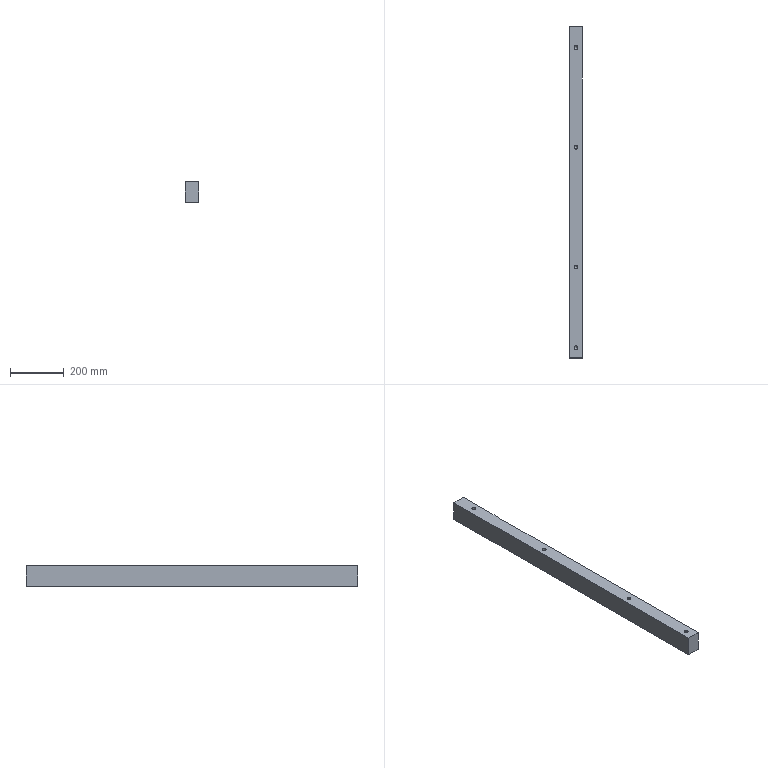Part | NX | features 3 2 | 1 solid | 24 faces | box 50 x 1233 x 75.5 mm | volume 4639640 mm3 | cylinder 9 | cone 8 | plane 7 | commonest cylinder face diameters 14.1 x8 54 x1
STEP:
#1=CARTESIAN_POINT('',(937.05,-522.5,256.5));
#2=VERTEX_POINT('',#1);
#3=CARTESIAN_POINT('',(930.,-522.5,256.5));
#4=DIRECTION('',(0.,0.,-1.));
#5=DIRECTION('',(1.,0.,0.));
#6=AXIS2_PLACEMENT_3D('',#3,#4,#5);
#7=CIRCLE('',#6,7.05);
#8=EDGE_CURVE('',#2,#2,#7,.T.);
#9=ORIENTED_EDGE('',*,*,#8,.T.);
#10=EDGE_LOOP('',(#9));
#11=FACE_BOUND('',#10,.T.);
#12=CARTESIAN_POINT('',(937.05,222.5,256.5));
#13=VERTEX_POINT('',#12);
#14=CARTESIAN_POINT('',(930.,222.5,256.5));
#15=DIRECTION('',(0.,0.,-1.));
#16=DIRECTION('',(1.,0.,0.));
#17=AXIS2_PLACEMENT_3D('',#14,#15,#16);
#18=CIRCLE('',#17,7.05);
#19=EDGE_CURVE('',#13,#13,#18,.T.);
#20=ORIENTED_EDGE('',*,*,#19,.T.);
#21=EDGE_LOOP('',(#20));
#22=FACE_BOUND('',#21,.T.);
#23=CARTESIAN_POINT('',(955.,469.802,256.5));
#24=VERTEX_POINT('',#23);
#25=CARTESIAN_POINT('',(955.,490.198,256.5));
#26=VERTEX_POINT('',#25);
#27=CARTESIAN_POINT('',(980.,480.,256.5));
#28=DIRECTION('',(0.,0.,-1.));
#29=DIRECTION('',(1.,0.,0.));
#30=AXIS2_PLACEMENT_3D('',#27,#28,#29);
#31=CIRCLE('',#30,27.);
#32=EDGE_CURVE('',#24,#26,#31,.T.);
#33=ORIENTED_EDGE('',*,*,#32,.T.);
#34=CARTESIAN_POINT('',(955.,672.5,256.5));
#35=VERTEX_POINT('',#34);
#36=CARTESIAN_POINT('',(955.,193.,256.5));
#37=DIRECTION('',(0.,-1.,0.));
#38=VECTOR('',#37,1000.);
#39=LINE('',#36,#38);
#40=EDGE_CURVE('',#35,#26,#39,.T.);
#41=ORIENTED_EDGE('',*,*,#40,.F.);
#42=CARTESIAN_POINT('',(905.,672.5,256.5));
#43=VERTEX_POINT('',#42);
#44=CARTESIAN_POINT('',(905.,672.5,256.5));
#45=DIRECTION('',(1.,0.,0.));
#46=VECTOR('',#45,1000.);
#47=LINE('',#44,#46);
#48=EDGE_CURVE('',#43,#35,#47,.T.);
#49=ORIENTED_EDGE('',*,*,#48,.F.);
#50=CARTESIAN_POINT('',(905.,-560.5,256.5));
#51=VERTEX_POINT('',#50);
#52=CARTESIAN_POINT('',(905.,193.,256.5));
#53=DIRECTION('',(0.,1.,0.));
#54=VECTOR('',#53,1000.);
#55=LINE('',#52,#54);
#56=EDGE_CURVE('',#51,#43,#55,.T.);
#57=ORIENTED_EDGE('',*,*,#56,.F.);
#58=CARTESIAN_POINT('',(955.,-560.5,256.5));
#59=VERTEX_POINT('',#58);
#60=CARTESIAN_POINT('',(2945.,-560.5,256.5));
#61=DIRECTION('',(1.,0.,0.));
#62=VECTOR('',#61,1000.);
#63=LINE('',#60,#62);
#64=EDGE_CURVE('',#51,#59,#63,.T.);
#65=ORIENTED_EDGE('',*,*,#64,.T.);
#66=CARTESIAN_POINT('',(955.,193.,256.5));
#67=DIRECTION('',(0.,-1.,0.));
#68=VECTOR('',#67,1000.);
#69=LINE('',#66,#68);
#70=EDGE_CURVE('',#24,#59,#69,.T.);
#71=ORIENTED_EDGE('',*,*,#70,.F.);
#72=EDGE_LOOP('',(#33,#41,#49,#57,#65,#71));
#73=FACE_BOUND('',#72,.T.);
#74=CARTESIAN_POINT('',(937.05,-222.5,256.5));
#75=VERTEX_POINT('',#74);
#76=CARTESIAN_POINT('',(930.,-222.5,256.5));
#77=DIRECTION('',(0.,0.,-1.));
#78=DIRECTION('',(1.,0.,0.));
#79=AXIS2_PLACEMENT_3D('',#76,#77,#78);
#80=CIRCLE('',#79,7.05);
#81=EDGE_CURVE('',#75,#75,#80,.T.);
#82=ORIENTED_EDGE('',*,*,#81,.T.);
#83=EDGE_LOOP('',(#82));
#84=FACE_BOUND('',#83,.T.);
#85=CARTESIAN_POINT('',(937.05,592.5,256.5));
#86=VERTEX_POINT('',#85);
#87=CARTESIAN_POINT('',(930.,592.5,256.5));
#88=DIRECTION('',(0.,0.,-1.));
#89=DIRECTION('',(1.,0.,0.));
#90=AXIS2_PLACEMENT_3D('',#87,#88,#89);
#91=CIRCLE('',#90,7.05);
#92=EDGE_CURVE('',#86,#86,#91,.T.);
#93=ORIENTED_EDGE('',*,*,#92,.T.);
#94=EDGE_LOOP('',(#93));
#95=FACE_BOUND('',#94,.T.);
#96=CARTESIAN_POINT('',(2945.,0.,256.5));
#97=DIRECTION('',(0.,0.,1.));
#98=DIRECTION('',(-1.,0.,0.));
#99=AXIS2_PLACEMENT_3D('',#96,#97,#98);
#100=PLANE('',#99);
#101=ADVANCED_FACE('',(#11,#22,#73,#84,#95),#100,.T.);
#102=CARTESIAN_POINT('',(937.05,222.5,181.));
#103=VERTEX_POINT('',#102);
#104=CARTESIAN_POINT('',(930.,222.5,181.));
#105=DIRECTION('',(0.,0.,1.));
#106=DIRECTION('',(1.,0.,0.));
#107=AXIS2_PLACEMENT_3D('',#104,#105,#106);
#108=CIRCLE('',#107,7.05);
#109=EDGE_CURVE('',#103,#103,#108,.T.);
#110=ORIENTED_EDGE('',*,*,#109,.T.);
#111=EDGE_LOOP('',(#110));
#112=FACE_BOUND('',#111,.T.);
#113=CARTESIAN_POINT('',(937.05,-222.5,181.));
#114=VERTEX_POINT('',#113);
#115=CARTESIAN_POINT('',(930.,-222.5,181.));
#116=DIRECTION('',(0.,0.,1.));
#117=DIRECTION('',(1.,0.,0.));
#118=AXIS2_PLACEMENT_3D('',#115,#116,#117);
#119=CIRCLE('',#118,7.05);
#120=EDGE_CURVE('',#114,#114,#119,.T.);
#121=ORIENTED_EDGE('',*,*,#120,.T.);
#122=EDGE_LOOP('',(#121));
#123=FACE_BOUND('',#122,.T.);
#124=CARTESIAN_POINT('',(955.,490.198,181.));
#125=VERTEX_POINT('',#124);
#126=CARTESIAN_POINT('',(955.,469.802,181.));
#127=VERTEX_POINT('',#126);
#128=CARTESIAN_POINT('',(980.,480.,181.));
#129=DIRECTION('',(0.,0.,1.));
#130=DIRECTION('',(-1.,0.,0.));
#131=AXIS2_PLACEMENT_3D('',#128,#129,#130);
#132=CIRCLE('',#131,27.);
#133=EDGE_CURVE('',#125,#127,#132,.T.);
#134=ORIENTED_EDGE('',*,*,#133,.T.);
#135=CARTESIAN_POINT('',(955.,-560.5,181.));
#136=VERTEX_POINT('',#135);
#137=CARTESIAN_POINT('',(955.,193.,181.));
#138=DIRECTION('',(0.,1.,0.));
#139=VECTOR('',#138,1000.);
#140=LINE('',#137,#139);
#141=EDGE_CURVE('',#136,#127,#140,.T.);
#142=ORIENTED_EDGE('',*,*,#141,.F.);
#143=CARTESIAN_POINT('',(905.,-560.5,181.));
#144=VERTEX_POINT('',#143);
#145=CARTESIAN_POINT('',(2175.,-560.5,181.));
#146=DIRECTION('',(-1.,0.,0.));
#147=VECTOR('',#146,1000.);
#148=LINE('',#145,#147);
#149=EDGE_CURVE('',#136,#144,#148,.T.);
#150=ORIENTED_EDGE('',*,*,#149,.T.);
#151=CARTESIAN_POINT('',(905.,672.5,181.));
#152=VERTEX_POINT('',#151);
#153=CARTESIAN_POINT('',(905.,193.,181.));
#154=DIRECTION('',(0.,-1.,0.));
#155=VECTOR('',#154,1000.);
#156=LINE('',#153,#155);
#157=EDGE_CURVE('',#152,#144,#156,.T.);
#158=ORIENTED_EDGE('',*,*,#157,.F.);
#159=CARTESIAN_POINT('',(955.,672.5,181.));
#160=VERTEX_POINT('',#159);
#161=CARTESIAN_POINT('',(2175.,672.5,181.));
#162=DIRECTION('',(1.,0.,0.));
#163=VECTOR('',#162,1000.);
#164=LINE('',#161,#163);
#165=EDGE_CURVE('',#152,#160,#164,.T.);
#166=ORIENTED_EDGE('',*,*,#165,.T.);
#167=CARTESIAN_POINT('',(955.,193.,181.));
#168=DIRECTION('',(0.,1.,0.));
#169=VECTOR('',#168,1000.);
#170=LINE('',#167,#169);
#171=EDGE_CURVE('',#125,#160,#170,.T.);
#172=ORIENTED_EDGE('',*,*,#171,.F.);
#173=EDGE_LOOP('',(#134,#142,#150,#158,#166,#172));
#174=FACE_BOUND('',#173,.T.);
#175=CARTESIAN_POINT('',(937.05,-522.5,181.));
#176=VERTEX_POINT('',#175);
#177=CARTESIAN_POINT('',(930.,-522.5,181.));
#178=DIRECTION('',(0.,0.,1.));
#179=DIRECTION('',(1.,0.,0.));
#180=AXIS2_PLACEMENT_3D('',#177,#178,#179);
#181=CIRCLE('',#180,7.05);
#182=EDGE_CURVE('',#176,#176,#181,.T.);
#183=ORIENTED_EDGE('',*,*,#182,.T.);
#184=EDGE_LOOP('',(#183));
#185=FACE_BOUND('',#184,.T.);
#186=CARTESIAN_POINT('',(937.05,592.5,181.));
#187=VERTEX_POINT('',#186);
#188=CARTESIAN_POINT('',(930.,592.5,181.));
#189=DIRECTION('',(0.,0.,1.));
#190=DIRECTION('',(1.,0.,0.));
#191=AXIS2_PLACEMENT_3D('',#188,#189,#190);
#192=CIRCLE('',#191,7.05);
#193=EDGE_CURVE('',#187,#187,#192,.T.);
#194=ORIENTED_EDGE('',*,*,#193,.T.);
#195=EDGE_LOOP('',(#194));
#196=FACE_BOUND('',#195,.T.);
#197=CARTESIAN_POINT('',(2175.,193.,181.));
#198=DIRECTION('',(0.,0.,-1.));
#199=DIRECTION('',(-1.,0.,0.));
#200=AXIS2_PLACEMENT_3D('',#197,#198,#199);
#201=PLANE('',#200);
#202=ADVANCED_FACE('',(#112,#123,#174,#185,#196),#201,.T.);
#203=CARTESIAN_POINT('',(955.,490.198,-181.));
#204=DIRECTION('',(0.,0.,1.));
#205=VECTOR('',#204,1000.);
#206=LINE('',#203,#205);
#207=EDGE_CURVE('',#125,#26,#206,.T.);
#208=ORIENTED_EDGE('',*,*,#207,.F.);
#209=ORIENTED_EDGE('',*,*,#171,.T.);
#210=CARTESIAN_POINT('',(955.,672.5,-1.5));
#211=DIRECTION('',(0.,0.,1.));
#212=VECTOR('',#211,1000.);
#213=LINE('',#210,#212);
#214=EDGE_CURVE('',#160,#35,#213,.T.);
#215=ORIENTED_EDGE('',*,*,#214,.T.);
#216=ORIENTED_EDGE('',*,*,#40,.T.);
#217=EDGE_LOOP('',(#208,#209,#215,#216));
#218=FACE_BOUND('',#217,.T.);
#219=CARTESIAN_POINT('',(955.,193.,-1.5));
#220=DIRECTION('',(1.,0.,0.));
#221=DIRECTION('',(0.,0.,1.));
#222=AXIS2_PLACEMENT_3D('',#219,#220,#221);
#223=PLANE('',#222);
#224=ADVANCED_FACE('',(#218),#223,.T.);
#225=ORIENTED_EDGE('',*,*,#64,.F.);
#226=CARTESIAN_POINT('',(905.,-560.5,-1.5));
#227=DIRECTION('',(0.,0.,1.));
#228=VECTOR('',#227,1000.);
#229=LINE('',#226,#228);
#230=EDGE_CURVE('',#144,#51,#229,.T.);
#231=ORIENTED_EDGE('',*,*,#230,.F.);
#232=ORIENTED_EDGE('',*,*,#149,.F.);
#233=CARTESIAN_POINT('',(955.,-560.5,-1.5));
#234=DIRECTION('',(0.,0.,-1.));
#235=VECTOR('',#234,1000.);
#236=LINE('',#233,#235);
#237=EDGE_CURVE('',#59,#136,#236,.T.);
#238=ORIENTED_EDGE('',*,*,#237,.F.);
#239=EDGE_LOOP('',(#225,#231,#232,#238));
#240=FACE_BOUND('',#239,.T.);
#241=CARTESIAN_POINT('',(903.,-560.5,179.));
#242=DIRECTION('',(0.,-1.,0.));
#243=DIRECTION('',(-1.,0.,0.));
#244=AXIS2_PLACEMENT_3D('',#241,#242,#243);
#245=PLANE('',#244);
#246=ADVANCED_FACE('',(#240),#245,.T.);
#247=ORIENTED_EDGE('',*,*,#157,.T.);
#248=ORIENTED_EDGE('',*,*,#230,.T.);
#249=ORIENTED_EDGE('',*,*,#56,.T.);
#250=CARTESIAN_POINT('',(905.,672.5,-1.5));
#251=DIRECTION('',(0.,0.,-1.));
#252=VECTOR('',#251,1000.);
#253=LINE('',#250,#252);
#254=EDGE_CURVE('',#43,#152,#253,.T.);
#255=ORIENTED_EDGE('',*,*,#254,.T.);
#256=EDGE_LOOP('',(#247,#248,#249,#255));
#257=FACE_BOUND('',#256,.T.);
#258=CARTESIAN_POINT('',(905.,193.,-1.5));
#259=DIRECTION('',(-1.,0.,0.));
#260=DIRECTION('',(0.,0.,-1.));
#261=AXIS2_PLACEMENT_3D('',#258,#259,#260);
#262=PLANE('',#261);
#263=ADVANCED_FACE('',(#257),#262,.T.);
#264=CARTESIAN_POINT('',(955.,469.802,256.5));
#265=DIRECTION('',(0.,0.,-1.));
#266=VECTOR('',#265,1000.);
#267=LINE('',#264,#266);
#268=EDGE_CURVE('',#24,#127,#267,.T.);
#269=ORIENTED_EDGE('',*,*,#268,.F.);
#270=ORIENTED_EDGE('',*,*,#70,.T.);
#271=ORIENTED_EDGE('',*,*,#237,.T.);
#272=ORIENTED_EDGE('',*,*,#141,.T.);
#273=EDGE_LOOP('',(#269,#270,#271,#272));
#274=FACE_BOUND('',#273,.T.);
#275=CARTESIAN_POINT('',(955.,193.,-1.5));
#276=DIRECTION('',(1.,0.,0.));
#277=DIRECTION('',(0.,0.,1.));
#278=AXIS2_PLACEMENT_3D('',#275,#276,#277);
#279=PLANE('',#278);
#280=ADVANCED_FACE('',(#274),#279,.T.);
#281=ORIENTED_EDGE('',*,*,#254,.F.);
#282=ORIENTED_EDGE('',*,*,#48,.T.);
#283=ORIENTED_EDGE('',*,*,#214,.F.);
#284=ORIENTED_EDGE('',*,*,#165,.F.);
#285=EDGE_LOOP('',(#281,#282,#283,#284));
#286=FACE_BOUND('',#285,.T.);
#287=CARTESIAN_POINT('',(905.,672.5,231.5));
#288=DIRECTION('',(0.,1.,0.));
#289=DIRECTION('',(0.,0.,-1.));
#290=AXIS2_PLACEMENT_3D('',#287,#288,#289);
#291=PLANE('',#290);
#292=ADVANCED_FACE('',(#286),#291,.T.);
#293=ORIENTED_EDGE('',*,*,#32,.F.);
#294=ORIENTED_EDGE('',*,*,#268,.T.);
#295=ORIENTED_EDGE('',*,*,#133,.F.);
#296=ORIENTED_EDGE('',*,*,#207,.T.);
#297=EDGE_LOOP('',(#293,#294,#295,#296));
#298=FACE_BOUND('',#297,.T.);
#299=CARTESIAN_POINT('',(980.,480.,-181.));
#300=DIRECTION('',(0.,0.,1.));
#301=DIRECTION('',(-1.,0.,0.));
#302=AXIS2_PLACEMENT_3D('',#299,#300,#301);
#303=CYLINDRICAL_SURFACE('',#302,27.);
#304=ADVANCED_FACE('',(#298),#303,.F.);
#305=CARTESIAN_POINT('',(937.05,-222.5,188.95));
#306=VERTEX_POINT('',#305);
#307=CARTESIAN_POINT('',(930.,-222.5,188.95));
#308=DIRECTION('',(0.,0.,1.));
#309=DIRECTION('',(1.,0.,0.));
#310=AXIS2_PLACEMENT_3D('',#307,#308,#309);
#311=CIRCLE('',#310,7.05);
#312=EDGE_CURVE('',#306,#306,#311,.T.);
#313=ORIENTED_EDGE('',*,*,#312,.T.);
#314=EDGE_LOOP('',(#313));
#315=FACE_BOUND('',#314,.T.);
#316=ORIENTED_EDGE('',*,*,#120,.F.);
#317=EDGE_LOOP('',(#316));
#318=FACE_BOUND('',#317,.T.);
#319=CARTESIAN_POINT('',(930.,-222.5,181.));
#320=DIRECTION('',(0.,0.,1.));
#321=DIRECTION('',(-1.,0.,0.));
#322=AXIS2_PLACEMENT_3D('',#319,#320,#321);
#323=CYLINDRICAL_SURFACE('',#322,7.05);
#324=ADVANCED_FACE('',(#315,#318),#323,.F.);
#325=CARTESIAN_POINT('',(930.,-222.5,196.));
#326=VERTEX_POINT('',#325);
#327=VERTEX_LOOP('',#326);
#328=FACE_BOUND('',#327,.T.);
#329=ORIENTED_EDGE('',*,*,#312,.F.);
#330=EDGE_LOOP('',(#329));
#331=FACE_BOUND('',#330,.T.);
#332=CARTESIAN_POINT('',(930.,-222.5,188.95));
#333=DIRECTION('',(0.,0.,-1.));
#334=DIRECTION('',(1.,0.,0.));
#335=AXIS2_PLACEMENT_3D('',#332,#333,#334);
#336=CONICAL_SURFACE('',#335,7.05,0.7854);
#337=ADVANCED_FACE('',(#328,#331),#336,.F.);
#338=CARTESIAN_POINT('',(937.05,-522.5,188.95));
#339=VERTEX_POINT('',#338);
#340=CARTESIAN_POINT('',(930.,-522.5,188.95));
#341=DIRECTION('',(0.,0.,1.));
#342=DIRECTION('',(1.,0.,0.));
#343=AXIS2_PLACEMENT_3D('',#340,#341,#342);
#344=CIRCLE('',#343,7.05);
#345=EDGE_CURVE('',#339,#339,#344,.T.);
#346=ORIENTED_EDGE('',*,*,#345,.T.);
#347=EDGE_LOOP('',(#346));
#348=FACE_BOUND('',#347,.T.);
#349=ORIENTED_EDGE('',*,*,#182,.F.);
#350=EDGE_LOOP('',(#349));
#351=FACE_BOUND('',#350,.T.);
#352=CARTESIAN_POINT('',(930.,-522.5,181.));
#353=DIRECTION('',(0.,0.,1.));
#354=DIRECTION('',(-1.,0.,0.));
#355=AXIS2_PLACEMENT_3D('',#352,#353,#354);
#356=CYLINDRICAL_SURFACE('',#355,7.05);
#357=ADVANCED_FACE('',(#348,#351),#356,.F.);
#358=CARTESIAN_POINT('',(930.,-522.5,196.));
#359=VERTEX_POINT('',#358);
#360=VERTEX_LOOP('',#359);
#361=FACE_BOUND('',#360,.T.);
#362=ORIENTED_EDGE('',*,*,#345,.F.);
#363=EDGE_LOOP('',(#362));
#364=FACE_BOUND('',#363,.T.);
#365=CARTESIAN_POINT('',(930.,-522.5,188.95));
#366=DIRECTION('',(0.,0.,-1.));
#367=DIRECTION('',(1.,0.,0.));
#368=AXIS2_PLACEMENT_3D('',#365,#366,#367);
#369=CONICAL_SURFACE('',#368,7.05,0.7854);
#370=ADVANCED_FACE('',(#361,#364),#369,.F.);
#371=CARTESIAN_POINT('',(937.05,222.5,188.95));
#372=VERTEX_POINT('',#371);
#373=CARTESIAN_POINT('',(930.,222.5,188.95));
#374=DIRECTION('',(0.,0.,1.));
#375=DIRECTION('',(1.,0.,0.));
#376=AXIS2_PLACEMENT_3D('',#373,#374,#375);
#377=CIRCLE('',#376,7.05);
#378=EDGE_CURVE('',#372,#372,#377,.T.);
#379=ORIENTED_EDGE('',*,*,#378,.T.);
#380=EDGE_LOOP('',(#379));
#381=FACE_BOUND('',#380,.T.);
#382=ORIENTED_EDGE('',*,*,#109,.F.);
#383=EDGE_LOOP('',(#382));
#384=FACE_BOUND('',#383,.T.);
#385=CARTESIAN_POINT('',(930.,222.5,181.));
#386=DIRECTION('',(0.,0.,1.));
#387=DIRECTION('',(-1.,0.,0.));
#388=AXIS2_PLACEMENT_3D('',#385,#386,#387);
#389=CYLINDRICAL_SURFACE('',#388,7.05);
#390=ADVANCED_FACE('',(#381,#384),#389,.F.);
#391=CARTESIAN_POINT('',(930.,222.5,196.));
#392=VERTEX_POINT('',#391);
#393=VERTEX_LOOP('',#392);
#394=FACE_BOUND('',#393,.T.);
#395=ORIENTED_EDGE('',*,*,#378,.F.);
#396=EDGE_LOOP('',(#395));
#397=FACE_BOUND('',#396,.T.);
#398=CARTESIAN_POINT('',(930.,222.5,188.95));
#399=DIRECTION('',(0.,0.,-1.));
#400=DIRECTION('',(1.,0.,0.));
#401=AXIS2_PLACEMENT_3D('',#398,#399,#400);
#402=CONICAL_SURFACE('',#401,7.05,0.7854);
#403=ADVANCED_FACE('',(#394,#397),#402,.F.);
#404=CARTESIAN_POINT('',(937.05,592.5,188.95));
#405=VERTEX_POINT('',#404);
#406=CARTESIAN_POINT('',(930.,592.5,188.95));
#407=DIRECTION('',(0.,0.,1.));
#408=DIRECTION('',(1.,0.,0.));
#409=AXIS2_PLACEMENT_3D('',#406,#407,#408);
#410=CIRCLE('',#409,7.05);
#411=EDGE_CURVE('',#405,#405,#410,.T.);
#412=ORIENTED_EDGE('',*,*,#411,.T.);
#413=EDGE_LOOP('',(#412));
#414=FACE_BOUND('',#413,.T.);
#415=ORIENTED_EDGE('',*,*,#193,.F.);
#416=EDGE_LOOP('',(#415));
#417=FACE_BOUND('',#416,.T.);
#418=CARTESIAN_POINT('',(930.,592.5,181.));
#419=DIRECTION('',(0.,0.,1.));
#420=DIRECTION('',(-1.,0.,0.));
#421=AXIS2_PLACEMENT_3D('',#418,#419,#420);
#422=CYLINDRICAL_SURFACE('',#421,7.05);
#423=ADVANCED_FACE('',(#414,#417),#422,.F.);
#424=CARTESIAN_POINT('',(930.,592.5,196.));
#425=VERTEX_POINT('',#424);
#426=VERTEX_LOOP('',#425);
#427=FACE_BOUND('',#426,.T.);
#428=ORIENTED_EDGE('',*,*,#411,.F.);
#429=EDGE_LOOP('',(#428));
#430=FACE_BOUND('',#429,.T.);
#431=CARTESIAN_POINT('',(930.,592.5,188.95));
#432=DIRECTION('',(0.,0.,-1.));
#433=DIRECTION('',(1.,0.,0.));
#434=AXIS2_PLACEMENT_3D('',#431,#432,#433);
#435=CONICAL_SURFACE('',#434,7.05,0.7854);
#436=ADVANCED_FACE('',(#427,#430),#435,.F.);
#437=CARTESIAN_POINT('',(922.95,222.5,248.55));
#438=VERTEX_POINT('',#437);
#439=CARTESIAN_POINT('',(930.,222.5,248.55));
#440=DIRECTION('',(0.,0.,-1.));
#441=DIRECTION('',(-1.,0.,0.));
#442=AXIS2_PLACEMENT_3D('',#439,#440,#441);
#443=CIRCLE('',#442,7.05);
#444=EDGE_CURVE('',#438,#438,#443,.T.);
#445=ORIENTED_EDGE('',*,*,#444,.T.);
#446=EDGE_LOOP('',(#445));
#447=FACE_BOUND('',#446,.T.);
#448=ORIENTED_EDGE('',*,*,#19,.F.);
#449=EDGE_LOOP('',(#448));
#450=FACE_BOUND('',#449,.T.);
#451=CARTESIAN_POINT('',(930.,222.5,256.5));
#452=DIRECTION('',(0.,0.,-1.));
#453=DIRECTION('',(-1.,0.,0.));
#454=AXIS2_PLACEMENT_3D('',#451,#452,#453);
#455=CYLINDRICAL_SURFACE('',#454,7.05);
#456=ADVANCED_FACE('',(#447,#450),#455,.F.);
#457=CARTESIAN_POINT('',(930.,222.5,241.5));
#458=VERTEX_POINT('',#457);
#459=VERTEX_LOOP('',#458);
#460=FACE_BOUND('',#459,.T.);
#461=ORIENTED_EDGE('',*,*,#444,.F.);
#462=EDGE_LOOP('',(#461));
#463=FACE_BOUND('',#462,.T.);
#464=CARTESIAN_POINT('',(930.,222.5,248.55));
#465=DIRECTION('',(0.,0.,1.));
#466=DIRECTION('',(-1.,0.,0.));
#467=AXIS2_PLACEMENT_3D('',#464,#465,#466);
#468=CONICAL_SURFACE('',#467,7.05,0.7854);
#469=ADVANCED_FACE('',(#460,#463),#468,.F.);
#470=CARTESIAN_POINT('',(922.95,-222.5,248.55));
#471=VERTEX_POINT('',#470);
#472=CARTESIAN_POINT('',(930.,-222.5,248.55));
#473=DIRECTION('',(0.,0.,-1.));
#474=DIRECTION('',(-1.,0.,0.));
#475=AXIS2_PLACEMENT_3D('',#472,#473,#474);
#476=CIRCLE('',#475,7.05);
#477=EDGE_CURVE('',#471,#471,#476,.T.);
#478=ORIENTED_EDGE('',*,*,#477,.T.);
#479=EDGE_LOOP('',(#478));
#480=FACE_BOUND('',#479,.T.);
#481=ORIENTED_EDGE('',*,*,#81,.F.);
#482=EDGE_LOOP('',(#481));
#483=FACE_BOUND('',#482,.T.);
#484=CARTESIAN_POINT('',(930.,-222.5,256.5));
#485=DIRECTION('',(0.,0.,-1.));
#486=DIRECTION('',(-1.,0.,0.));
#487=AXIS2_PLACEMENT_3D('',#484,#485,#486);
#488=CYLINDRICAL_SURFACE('',#487,7.05);
#489=ADVANCED_FACE('',(#480,#483),#488,.F.);
#490=CARTESIAN_POINT('',(930.,-222.5,241.5));
#491=VERTEX_POINT('',#490);
#492=VERTEX_LOOP('',#491);
#493=FACE_BOUND('',#492,.T.);
#494=ORIENTED_EDGE('',*,*,#477,.F.);
#495=EDGE_LOOP('',(#494));
#496=FACE_BOUND('',#495,.T.);
#497=CARTESIAN_POINT('',(930.,-222.5,248.55));
#498=DIRECTION('',(0.,0.,1.));
#499=DIRECTION('',(-1.,0.,0.));
#500=AXIS2_PLACEMENT_3D('',#497,#498,#499);
#501=CONICAL_SURFACE('',#500,7.05,0.7854);
#502=ADVANCED_FACE('',(#493,#496),#501,.F.);
#503=CARTESIAN_POINT('',(922.95,-522.5,248.55));
#504=VERTEX_POINT('',#503);
#505=CARTESIAN_POINT('',(930.,-522.5,248.55));
#506=DIRECTION('',(0.,0.,-1.));
#507=DIRECTION('',(-1.,0.,0.));
#508=AXIS2_PLACEMENT_3D('',#505,#506,#507);
#509=CIRCLE('',#508,7.05);
#510=EDGE_CURVE('',#504,#504,#509,.T.);
#511=ORIENTED_EDGE('',*,*,#510,.T.);
#512=EDGE_LOOP('',(#511));
#513=FACE_BOUND('',#512,.T.);
#514=ORIENTED_EDGE('',*,*,#8,.F.);
#515=EDGE_LOOP('',(#514));
#516=FACE_BOUND('',#515,.T.);
#517=CARTESIAN_POINT('',(930.,-522.5,256.5));
#518=DIRECTION('',(0.,0.,-1.));
#519=DIRECTION('',(-1.,0.,0.));
#520=AXIS2_PLACEMENT_3D('',#517,#518,#519);
#521=CYLINDRICAL_SURFACE('',#520,7.05);
#522=ADVANCED_FACE('',(#513,#516),#521,.F.);
#523=CARTESIAN_POINT('',(930.,-522.5,241.5));
#524=VERTEX_POINT('',#523);
#525=VERTEX_LOOP('',#524);
#526=FACE_BOUND('',#525,.T.);
#527=ORIENTED_EDGE('',*,*,#510,.F.);
#528=EDGE_LOOP('',(#527));
#529=FACE_BOUND('',#528,.T.);
#530=CARTESIAN_POINT('',(930.,-522.5,248.55));
#531=DIRECTION('',(0.,0.,1.));
#532=DIRECTION('',(-1.,0.,0.));
#533=AXIS2_PLACEMENT_3D('',#530,#531,#532);
#534=CONICAL_SURFACE('',#533,7.05,0.7854);
#535=ADVANCED_FACE('',(#526,#529),#534,.F.);
#536=CARTESIAN_POINT('',(922.95,592.5,248.55));
#537=VERTEX_POINT('',#536);
#538=CARTESIAN_POINT('',(930.,592.5,248.55));
#539=DIRECTION('',(0.,0.,-1.));
#540=DIRECTION('',(-1.,0.,0.));
#541=AXIS2_PLACEMENT_3D('',#538,#539,#540);
#542=CIRCLE('',#541,7.05);
#543=EDGE_CURVE('',#537,#537,#542,.T.);
#544=ORIENTED_EDGE('',*,*,#543,.T.);
#545=EDGE_LOOP('',(#544));
#546=FACE_BOUND('',#545,.T.);
#547=ORIENTED_EDGE('',*,*,#92,.F.);
#548=EDGE_LOOP('',(#547));
#549=FACE_BOUND('',#548,.T.);
#550=CARTESIAN_POINT('',(930.,592.5,256.5));
#551=DIRECTION('',(0.,0.,-1.));
#552=DIRECTION('',(-1.,0.,0.));
#553=AXIS2_PLACEMENT_3D('',#550,#551,#552);
#554=CYLINDRICAL_SURFACE('',#553,7.05);
#555=ADVANCED_FACE('',(#546,#549),#554,.F.);
#556=CARTESIAN_POINT('',(930.,592.5,241.5));
#557=VERTEX_POINT('',#556);
#558=VERTEX_LOOP('',#557);
#559=FACE_BOUND('',#558,.T.);
#560=ORIENTED_EDGE('',*,*,#543,.F.);
#561=EDGE_LOOP('',(#560));
#562=FACE_BOUND('',#561,.T.);
#563=CARTESIAN_POINT('',(930.,592.5,248.55));
#564=DIRECTION('',(0.,0.,1.));
#565=DIRECTION('',(-1.,0.,0.));
#566=AXIS2_PLACEMENT_3D('',#563,#564,#565);
#567=CONICAL_SURFACE('',#566,7.05,0.7854);
#568=ADVANCED_FACE('',(#559,#562),#567,.F.);
#569=CLOSED_SHELL('',(#101,#202,#224,#246,#263,#280,#292,#304,#324,#337,#357,#370,#390,#403,#423,#436,#456,#469,#489,#502,#522,#535,#555,#568));
#570=MANIFOLD_SOLID_BREP('',#569);
#571=(LENGTH_UNIT()NAMED_UNIT(*)SI_UNIT(.MILLI.,.METRE.));
#572=UNCERTAINTY_MEASURE_WITH_UNIT(LENGTH_MEASURE(0.00001),#571,'','');
#573=(NAMED_UNIT(*)PLANE_ANGLE_UNIT()SI_UNIT($,.RADIAN.));
#574=(NAMED_UNIT(*)SI_UNIT($,.STERADIAN.)SOLID_ANGLE_UNIT());
#575=(GEOMETRIC_REPRESENTATION_CONTEXT(3)GLOBAL_UNCERTAINTY_ASSIGNED_CONTEXT((#572))GLOBAL_UNIT_ASSIGNED_CONTEXT((#571,#573,#574))REPRESENTATION_CONTEXT('',''));
#576=ADVANCED_BREP_SHAPE_REPRESENTATION('',(#570),#575);